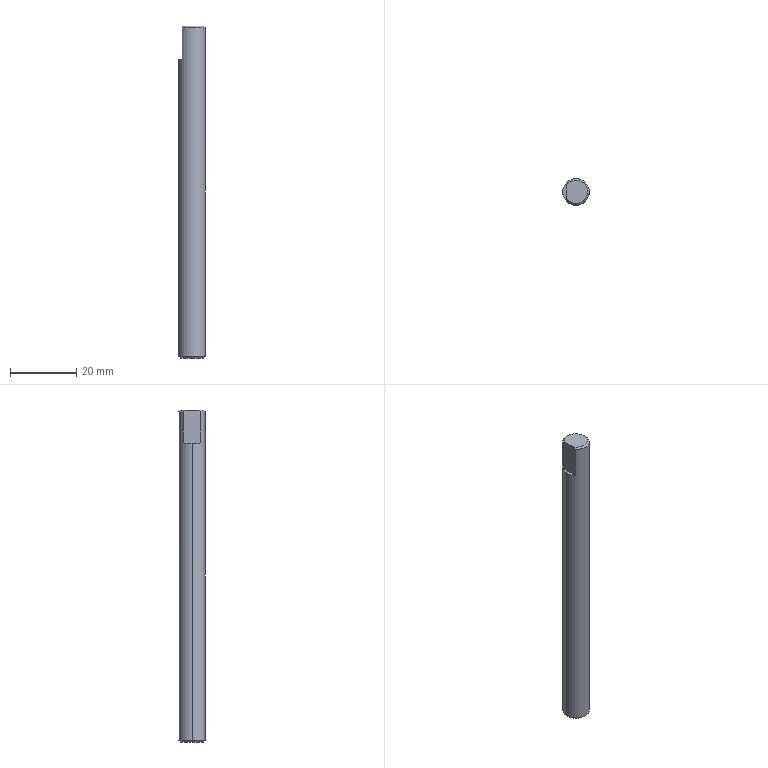Part | STEP file | positioning guide rod | 1 solid | 9 faces | box 8 x 8 x 100 mm | volume 4985 mm3 | plane 4 | cone 3 | cylinder 2 | commonest cylinder face diameters 8 x2
STEP:
#1=CARTESIAN_POINT('',(0.,0.,0.));
#2=DIRECTION('',(0.,0.,1.));
#3=DIRECTION('',(1.,0.,0.));
#4=AXIS2_PLACEMENT_3D('',#1,#2,#3);
#5=CARTESIAN_POINT('',(-3.5,0.,-50.));
#6=VERTEX_POINT('',#5);
#7=CARTESIAN_POINT('',(3.5,0.,-50.));
#8=VERTEX_POINT('',#7);
#9=CARTESIAN_POINT('',(0.,0.,-50.));
#10=DIRECTION('',(0.,0.,-1.));
#11=DIRECTION('',(1.,0.,0.));
#12=AXIS2_PLACEMENT_3D('',#9,#10,#11);
#13=CIRCLE('',#12,3.5);
#14=CARTESIAN_POINT('',(0.,0.,-49.5));
#15=DIRECTION('',(0.,0.,1.));
#16=DIRECTION('',(1.,0.,0.));
#17=AXIS2_PLACEMENT_3D('',#14,#15,#16);
#18=CONICAL_SURFACE('',#17,4.,0.7854);
#19=CARTESIAN_POINT('',(6.283,-0.5));
#20=DIRECTION('',(-1.,0.));
#21=VECTOR('',#20,1.);
#22=LINE('',#19,#21);
#23=(GEOMETRIC_REPRESENTATION_CONTEXT(2)PARAMETRIC_REPRESENTATION_CONTEXT()REPRESENTATION_CONTEXT('',''));
#24=DEFINITIONAL_REPRESENTATION('',(#22),#23);
#25=PCURVE('',#18,#24);
#26=CARTESIAN_POINT('',(0.,0.,-50.));
#27=DIRECTION('',(0.,0.,1.));
#28=DIRECTION('',(1.,0.,0.));
#29=AXIS2_PLACEMENT_3D('',#26,#27,#28);
#30=PLANE('',#29);
#31=CARTESIAN_POINT('',(3.5,0.));
#32=CARTESIAN_POINT('',(3.5,-6.062));
#33=CARTESIAN_POINT('',(-1.75,-3.031));
#34=CARTESIAN_POINT('',(-7.,0.));
#35=CARTESIAN_POINT('',(-1.75,3.031));
#36=CARTESIAN_POINT('',(3.5,6.062));
#37=CARTESIAN_POINT('',(3.5,0.));
#38=(BOUNDED_CURVE()B_SPLINE_CURVE(2,(#31,#32,#33,#34,#35,#36,#37),.UNSPECIFIED.,.T.,.F.)B_SPLINE_CURVE_WITH_KNOTS((1,2,2,2,2,1),(-2.094,0.,2.094,4.189,6.283,8.378),.UNSPECIFIED.)CURVE()GEOMETRIC_REPRESENTATION_ITEM()RATIONAL_B_SPLINE_CURVE((1.,0.5,1.,0.5,1.,0.5,1.))REPRESENTATION_ITEM(''));
#39=(GEOMETRIC_REPRESENTATION_CONTEXT(2)PARAMETRIC_REPRESENTATION_CONTEXT()REPRESENTATION_CONTEXT('',''));
#40=DEFINITIONAL_REPRESENTATION('',(#38),#39);
#41=PCURVE('',#30,#40);
#42=SURFACE_CURVE('',#13,(#25,#41),.PCURVE_S1.);
#43=EDGE_CURVE('',#6,#8,#42,.T.);
#44=ORIENTED_EDGE('',*,*,#43,.F.);
#45=CARTESIAN_POINT('',(-4.,0.,-49.5));
#46=VERTEX_POINT('',#45);
#47=CARTESIAN_POINT('',(-4.,0.,-49.5));
#48=DIRECTION('',(-0.7071,0.,0.7071));
#49=VECTOR('',#48,1.);
#50=LINE('',#47,#49);
#51=CARTESIAN_POINT('',(3.142,0.));
#52=DIRECTION('',(0.,1.));
#53=VECTOR('',#52,1.);
#54=LINE('',#51,#53);
#55=(GEOMETRIC_REPRESENTATION_CONTEXT(2)PARAMETRIC_REPRESENTATION_CONTEXT()REPRESENTATION_CONTEXT('',''));
#56=DEFINITIONAL_REPRESENTATION('',(#54),#55);
#57=PCURVE('',#18,#56);
#58=CARTESIAN_POINT('',(0.,0.,-49.5));
#59=DIRECTION('',(0.,0.,1.));
#60=DIRECTION('',(1.,0.,0.));
#61=AXIS2_PLACEMENT_3D('',#58,#59,#60);
#62=CONICAL_SURFACE('',#61,4.,0.7854);
#63=CARTESIAN_POINT('',(3.142,0.));
#64=DIRECTION('',(0.,1.));
#65=VECTOR('',#64,1.);
#66=LINE('',#63,#65);
#67=(GEOMETRIC_REPRESENTATION_CONTEXT(2)PARAMETRIC_REPRESENTATION_CONTEXT()REPRESENTATION_CONTEXT('',''));
#68=DEFINITIONAL_REPRESENTATION('',(#66),#67);
#69=PCURVE('',#62,#68);
#70=SURFACE_CURVE('',#50,(#57,#69),.PCURVE_S1.);
#71=EDGE_CURVE('',#6,#46,#70,.T.);
#72=ORIENTED_EDGE('',*,*,#71,.T.);
#73=CARTESIAN_POINT('',(4.,0.,-49.5));
#74=VERTEX_POINT('',#73);
#75=CARTESIAN_POINT('',(0.,0.,-49.5));
#76=DIRECTION('',(0.,0.,1.));
#77=DIRECTION('',(1.,0.,0.));
#78=AXIS2_PLACEMENT_3D('',#75,#76,#77);
#79=CIRCLE('',#78,4.);
#80=CARTESIAN_POINT('',(0.,0.));
#81=DIRECTION('',(1.,0.));
#82=VECTOR('',#81,1.);
#83=LINE('',#80,#82);
#84=(GEOMETRIC_REPRESENTATION_CONTEXT(2)PARAMETRIC_REPRESENTATION_CONTEXT()REPRESENTATION_CONTEXT('',''));
#85=DEFINITIONAL_REPRESENTATION('',(#83),#84);
#86=PCURVE('',#18,#85);
#87=CARTESIAN_POINT('',(0.,0.,50.));
#88=DIRECTION('',(0.,0.,-1.));
#89=DIRECTION('',(-1.,0.,0.));
#90=AXIS2_PLACEMENT_3D('',#87,#88,#89);
#91=CYLINDRICAL_SURFACE('',#90,4.);
#92=CARTESIAN_POINT('',(3.142,99.5));
#93=DIRECTION('',(-1.,0.));
#94=VECTOR('',#93,1.);
#95=LINE('',#92,#94);
#96=(GEOMETRIC_REPRESENTATION_CONTEXT(2)PARAMETRIC_REPRESENTATION_CONTEXT()REPRESENTATION_CONTEXT('',''));
#97=DEFINITIONAL_REPRESENTATION('',(#95),#96);
#98=PCURVE('',#91,#97);
#99=SURFACE_CURVE('',#79,(#86,#98),.PCURVE_S1.);
#100=EDGE_CURVE('',#74,#46,#99,.T.);
#101=ORIENTED_EDGE('',*,*,#100,.F.);
#102=CARTESIAN_POINT('',(4.,0.,-49.5));
#103=DIRECTION('',(0.7071,0.,0.7071));
#104=VECTOR('',#103,1.);
#105=LINE('',#102,#104);
#106=CARTESIAN_POINT('',(0.,0.));
#107=DIRECTION('',(0.,1.));
#108=VECTOR('',#107,1.);
#109=LINE('',#106,#108);
#110=(GEOMETRIC_REPRESENTATION_CONTEXT(2)PARAMETRIC_REPRESENTATION_CONTEXT()REPRESENTATION_CONTEXT('',''));
#111=DEFINITIONAL_REPRESENTATION('',(#109),#110);
#112=PCURVE('',#18,#111);
#113=CARTESIAN_POINT('',(6.283,0.));
#114=DIRECTION('',(0.,1.));
#115=VECTOR('',#114,1.);
#116=LINE('',#113,#115);
#117=(GEOMETRIC_REPRESENTATION_CONTEXT(2)PARAMETRIC_REPRESENTATION_CONTEXT()REPRESENTATION_CONTEXT('',''));
#118=DEFINITIONAL_REPRESENTATION('',(#116),#117);
#119=PCURVE('',#62,#118);
#120=SURFACE_CURVE('',#105,(#112,#119),.PCURVE_S1.);
#121=EDGE_CURVE('',#8,#74,#120,.T.);
#122=ORIENTED_EDGE('',*,*,#121,.F.);
#123=EDGE_LOOP('',(#44,#72,#101,#122));
#124=FACE_BOUND('',#123,.T.);
#125=ADVANCED_FACE('',(#124),#18,.T.);
#126=CARTESIAN_POINT('',(-3.,2.646,49.5));
#127=VERTEX_POINT('',#126);
#128=CARTESIAN_POINT('',(4.,0.,49.5));
#129=VERTEX_POINT('',#128);
#130=CARTESIAN_POINT('',(0.,0.,49.5));
#131=DIRECTION('',(0.,0.,-1.));
#132=DIRECTION('',(1.,0.,0.));
#133=AXIS2_PLACEMENT_3D('',#130,#131,#132);
#134=CIRCLE('',#133,4.);
#135=CARTESIAN_POINT('',(-3.142,0.5));
#136=DIRECTION('',(1.,0.));
#137=VECTOR('',#136,1.);
#138=LINE('',#135,#137);
#139=(GEOMETRIC_REPRESENTATION_CONTEXT(2)PARAMETRIC_REPRESENTATION_CONTEXT()REPRESENTATION_CONTEXT('',''));
#140=DEFINITIONAL_REPRESENTATION('',(#138),#139);
#141=PCURVE('',#91,#140);
#142=CARTESIAN_POINT('',(0.,0.,50.));
#143=DIRECTION('',(0.,0.,-1.));
#144=DIRECTION('',(-1.,0.,0.));
#145=AXIS2_PLACEMENT_3D('',#142,#143,#144);
#146=CONICAL_SURFACE('',#145,3.5,0.7854);
#147=CARTESIAN_POINT('',(-3.142,0.5));
#148=DIRECTION('',(1.,0.));
#149=VECTOR('',#148,1.);
#150=LINE('',#147,#149);
#151=(GEOMETRIC_REPRESENTATION_CONTEXT(2)PARAMETRIC_REPRESENTATION_CONTEXT()REPRESENTATION_CONTEXT('',''));
#152=DEFINITIONAL_REPRESENTATION('',(#150),#151);
#153=PCURVE('',#146,#152);
#154=SURFACE_CURVE('',#134,(#141,#153),.PCURVE_S1.);
#155=EDGE_CURVE('',#127,#129,#154,.T.);
#156=ORIENTED_EDGE('',*,*,#155,.T.);
#157=CARTESIAN_POINT('',(4.,0.,50.));
#158=DIRECTION('',(0.,0.,-1.));
#159=VECTOR('',#158,1.);
#160=LINE('',#157,#159);
#161=CARTESIAN_POINT('',(3.142,0.));
#162=DIRECTION('',(0.,1.));
#163=VECTOR('',#162,1.);
#164=LINE('',#161,#163);
#165=(GEOMETRIC_REPRESENTATION_CONTEXT(2)PARAMETRIC_REPRESENTATION_CONTEXT()REPRESENTATION_CONTEXT('',''));
#166=DEFINITIONAL_REPRESENTATION('',(#164),#165);
#167=PCURVE('',#91,#166);
#168=CARTESIAN_POINT('',(0.,0.,50.));
#169=DIRECTION('',(0.,0.,-1.));
#170=DIRECTION('',(-1.,0.,0.));
#171=AXIS2_PLACEMENT_3D('',#168,#169,#170);
#172=CYLINDRICAL_SURFACE('',#171,4.);
#173=CARTESIAN_POINT('',(3.142,0.));
#174=DIRECTION('',(0.,1.));
#175=VECTOR('',#174,1.);
#176=LINE('',#173,#175);
#177=(GEOMETRIC_REPRESENTATION_CONTEXT(2)PARAMETRIC_REPRESENTATION_CONTEXT()REPRESENTATION_CONTEXT('',''));
#178=DEFINITIONAL_REPRESENTATION('',(#176),#177);
#179=PCURVE('',#172,#178);
#180=SURFACE_CURVE('',#160,(#167,#179),.PCURVE_S1.);
#181=EDGE_CURVE('',#129,#74,#180,.T.);
#182=ORIENTED_EDGE('',*,*,#181,.T.);
#183=ORIENTED_EDGE('',*,*,#100,.T.);
#184=CARTESIAN_POINT('',(-4.,0.,40.));
#185=VERTEX_POINT('',#184);
#186=CARTESIAN_POINT('',(-4.,0.,50.));
#187=DIRECTION('',(0.,0.,-1.));
#188=VECTOR('',#187,1.);
#189=LINE('',#186,#188);
#190=CARTESIAN_POINT('',(0.,0.));
#191=DIRECTION('',(0.,1.));
#192=VECTOR('',#191,1.);
#193=LINE('',#190,#192);
#194=(GEOMETRIC_REPRESENTATION_CONTEXT(2)PARAMETRIC_REPRESENTATION_CONTEXT()REPRESENTATION_CONTEXT('',''));
#195=DEFINITIONAL_REPRESENTATION('',(#193),#194);
#196=PCURVE('',#91,#195);
#197=CARTESIAN_POINT('',(6.283,0.));
#198=DIRECTION('',(0.,1.));
#199=VECTOR('',#198,1.);
#200=LINE('',#197,#199);
#201=(GEOMETRIC_REPRESENTATION_CONTEXT(2)PARAMETRIC_REPRESENTATION_CONTEXT()REPRESENTATION_CONTEXT('',''));
#202=DEFINITIONAL_REPRESENTATION('',(#200),#201);
#203=PCURVE('',#172,#202);
#204=SURFACE_CURVE('',#189,(#196,#203),.PCURVE_S1.);
#205=EDGE_CURVE('',#185,#46,#204,.T.);
#206=ORIENTED_EDGE('',*,*,#205,.F.);
#207=CARTESIAN_POINT('',(-3.,2.646,40.));
#208=VERTEX_POINT('',#207);
#209=CARTESIAN_POINT('',(0.,0.,40.));
#210=DIRECTION('',(0.,0.,1.));
#211=DIRECTION('',(1.,0.,0.));
#212=AXIS2_PLACEMENT_3D('',#209,#210,#211);
#213=CIRCLE('',#212,4.);
#214=CARTESIAN_POINT('',(3.142,10.));
#215=DIRECTION('',(-1.,0.));
#216=VECTOR('',#215,1.);
#217=LINE('',#214,#216);
#218=(GEOMETRIC_REPRESENTATION_CONTEXT(2)PARAMETRIC_REPRESENTATION_CONTEXT()REPRESENTATION_CONTEXT('',''));
#219=DEFINITIONAL_REPRESENTATION('',(#217),#218);
#220=PCURVE('',#91,#219);
#221=CARTESIAN_POINT('',(0.,0.,40.));
#222=DIRECTION('',(0.,0.,1.));
#223=DIRECTION('',(1.,0.,0.));
#224=AXIS2_PLACEMENT_3D('',#221,#222,#223);
#225=PLANE('',#224);
#226=CARTESIAN_POINT('',(0.,0.));
#227=DIRECTION('',(1.,0.));
#228=AXIS2_PLACEMENT_2D('',#226,#227);
#229=CIRCLE('',#228,4.);
#230=(GEOMETRIC_REPRESENTATION_CONTEXT(2)PARAMETRIC_REPRESENTATION_CONTEXT()REPRESENTATION_CONTEXT('',''));
#231=DEFINITIONAL_REPRESENTATION('',(#229),#230);
#232=PCURVE('',#225,#231);
#233=SURFACE_CURVE('',#213,(#220,#232),.PCURVE_S1.);
#234=EDGE_CURVE('',#208,#185,#233,.T.);
#235=ORIENTED_EDGE('',*,*,#234,.F.);
#236=CARTESIAN_POINT('',(-3.,2.646,50.));
#237=DIRECTION('',(0.,0.,1.));
#238=VECTOR('',#237,1.);
#239=LINE('',#236,#238);
#240=CARTESIAN_POINT('',(0.7227,0.));
#241=DIRECTION('',(0.,-1.));
#242=VECTOR('',#241,1.);
#243=LINE('',#240,#242);
#244=(GEOMETRIC_REPRESENTATION_CONTEXT(2)PARAMETRIC_REPRESENTATION_CONTEXT()REPRESENTATION_CONTEXT('',''));
#245=DEFINITIONAL_REPRESENTATION('',(#243),#244);
#246=PCURVE('',#91,#245);
#247=CARTESIAN_POINT('',(-3.,2.975,40.));
#248=DIRECTION('',(1.,0.,0.));
#249=DIRECTION('',(0.,1.,0.));
#250=AXIS2_PLACEMENT_3D('',#247,#248,#249);
#251=PLANE('',#250);
#252=CARTESIAN_POINT('',(-0.329,10.));
#253=DIRECTION('',(0.,1.));
#254=VECTOR('',#253,1.);
#255=LINE('',#252,#254);
#256=(GEOMETRIC_REPRESENTATION_CONTEXT(2)PARAMETRIC_REPRESENTATION_CONTEXT()REPRESENTATION_CONTEXT('',''));
#257=DEFINITIONAL_REPRESENTATION('',(#255),#256);
#258=PCURVE('',#251,#257);
#259=SURFACE_CURVE('',#239,(#246,#258),.PCURVE_S1.);
#260=EDGE_CURVE('',#208,#127,#259,.T.);
#261=ORIENTED_EDGE('',*,*,#260,.T.);
#262=EDGE_LOOP('',(#156,#182,#183,#206,#235,#261));
#263=FACE_BOUND('',#262,.T.);
#264=ADVANCED_FACE('',(#263),#91,.T.);
#265=ORIENTED_EDGE('',*,*,#181,.F.);
#266=CARTESIAN_POINT('',(-3.,-2.646,49.5));
#267=VERTEX_POINT('',#266);
#268=CARTESIAN_POINT('',(0.,0.,49.5));
#269=DIRECTION('',(0.,0.,-1.));
#270=DIRECTION('',(1.,0.,0.));
#271=AXIS2_PLACEMENT_3D('',#268,#269,#270);
#272=CIRCLE('',#271,4.);
#273=CARTESIAN_POINT('',(3.142,0.5));
#274=DIRECTION('',(1.,0.));
#275=VECTOR('',#274,1.);
#276=LINE('',#273,#275);
#277=(GEOMETRIC_REPRESENTATION_CONTEXT(2)PARAMETRIC_REPRESENTATION_CONTEXT()REPRESENTATION_CONTEXT('',''));
#278=DEFINITIONAL_REPRESENTATION('',(#276),#277);
#279=PCURVE('',#172,#278);
#280=CARTESIAN_POINT('',(3.142,0.5));
#281=DIRECTION('',(1.,0.));
#282=VECTOR('',#281,1.);
#283=LINE('',#280,#282);
#284=(GEOMETRIC_REPRESENTATION_CONTEXT(2)PARAMETRIC_REPRESENTATION_CONTEXT()REPRESENTATION_CONTEXT('',''));
#285=DEFINITIONAL_REPRESENTATION('',(#283),#284);
#286=PCURVE('',#146,#285);
#287=SURFACE_CURVE('',#272,(#279,#286),.PCURVE_S1.);
#288=EDGE_CURVE('',#129,#267,#287,.T.);
#289=ORIENTED_EDGE('',*,*,#288,.T.);
#290=CARTESIAN_POINT('',(-3.,-2.646,40.));
#291=VERTEX_POINT('',#290);
#292=CARTESIAN_POINT('',(-3.,-2.646,50.));
#293=DIRECTION('',(0.,0.,-1.));
#294=VECTOR('',#293,1.);
#295=LINE('',#292,#294);
#296=CARTESIAN_POINT('',(5.56,0.));
#297=DIRECTION('',(0.,1.));
#298=VECTOR('',#297,1.);
#299=LINE('',#296,#298);
#300=(GEOMETRIC_REPRESENTATION_CONTEXT(2)PARAMETRIC_REPRESENTATION_CONTEXT()REPRESENTATION_CONTEXT('',''));
#301=DEFINITIONAL_REPRESENTATION('',(#299),#300);
#302=PCURVE('',#172,#301);
#303=CARTESIAN_POINT('',(-5.62,10.));
#304=DIRECTION('',(0.,-1.));
#305=VECTOR('',#304,1.);
#306=LINE('',#303,#305);
#307=(GEOMETRIC_REPRESENTATION_CONTEXT(2)PARAMETRIC_REPRESENTATION_CONTEXT()REPRESENTATION_CONTEXT('',''));
#308=DEFINITIONAL_REPRESENTATION('',(#306),#307);
#309=PCURVE('',#251,#308);
#310=SURFACE_CURVE('',#295,(#302,#309),.PCURVE_S1.);
#311=EDGE_CURVE('',#267,#291,#310,.T.);
#312=ORIENTED_EDGE('',*,*,#311,.T.);
#313=CARTESIAN_POINT('',(0.,0.,40.));
#314=DIRECTION('',(0.,0.,1.));
#315=DIRECTION('',(1.,0.,0.));
#316=AXIS2_PLACEMENT_3D('',#313,#314,#315);
#317=CIRCLE('',#316,4.);
#318=CARTESIAN_POINT('',(9.425,10.));
#319=DIRECTION('',(-1.,0.));
#320=VECTOR('',#319,1.);
#321=LINE('',#318,#320);
#322=(GEOMETRIC_REPRESENTATION_CONTEXT(2)PARAMETRIC_REPRESENTATION_CONTEXT()REPRESENTATION_CONTEXT('',''));
#323=DEFINITIONAL_REPRESENTATION('',(#321),#322);
#324=PCURVE('',#172,#323);
#325=CARTESIAN_POINT('',(0.,0.));
#326=DIRECTION('',(1.,0.));
#327=AXIS2_PLACEMENT_2D('',#325,#326);
#328=CIRCLE('',#327,4.);
#329=(GEOMETRIC_REPRESENTATION_CONTEXT(2)PARAMETRIC_REPRESENTATION_CONTEXT()REPRESENTATION_CONTEXT('',''));
#330=DEFINITIONAL_REPRESENTATION('',(#328),#329);
#331=PCURVE('',#225,#330);
#332=SURFACE_CURVE('',#317,(#324,#331),.PCURVE_S1.);
#333=EDGE_CURVE('',#185,#291,#332,.T.);
#334=ORIENTED_EDGE('',*,*,#333,.F.);
#335=ORIENTED_EDGE('',*,*,#205,.T.);
#336=CARTESIAN_POINT('',(0.,0.,-49.5));
#337=DIRECTION('',(0.,0.,1.));
#338=DIRECTION('',(1.,0.,0.));
#339=AXIS2_PLACEMENT_3D('',#336,#337,#338);
#340=CIRCLE('',#339,4.);
#341=CARTESIAN_POINT('',(9.425,99.5));
#342=DIRECTION('',(-1.,0.));
#343=VECTOR('',#342,1.);
#344=LINE('',#341,#343);
#345=(GEOMETRIC_REPRESENTATION_CONTEXT(2)PARAMETRIC_REPRESENTATION_CONTEXT()REPRESENTATION_CONTEXT('',''));
#346=DEFINITIONAL_REPRESENTATION('',(#344),#345);
#347=PCURVE('',#172,#346);
#348=CARTESIAN_POINT('',(0.,0.));
#349=DIRECTION('',(1.,0.));
#350=VECTOR('',#349,1.);
#351=LINE('',#348,#350);
#352=(GEOMETRIC_REPRESENTATION_CONTEXT(2)PARAMETRIC_REPRESENTATION_CONTEXT()REPRESENTATION_CONTEXT('',''));
#353=DEFINITIONAL_REPRESENTATION('',(#351),#352);
#354=PCURVE('',#62,#353);
#355=SURFACE_CURVE('',#340,(#347,#354),.PCURVE_S1.);
#356=EDGE_CURVE('',#46,#74,#355,.T.);
#357=ORIENTED_EDGE('',*,*,#356,.T.);
#358=EDGE_LOOP('',(#265,#289,#312,#334,#335,#357));
#359=FACE_BOUND('',#358,.T.);
#360=ADVANCED_FACE('',(#359),#172,.T.);
#361=CARTESIAN_POINT('',(-3.,-1.803,50.));
#362=VERTEX_POINT('',#361);
#363=CARTESIAN_POINT('',(-3.,1.803,50.));
#364=VERTEX_POINT('',#363);
#365=CARTESIAN_POINT('',(-3.,2.975,50.));
#366=DIRECTION('',(0.,1.,0.));
#367=VECTOR('',#366,1.);
#368=LINE('',#365,#367);
#369=CARTESIAN_POINT('',(0.,0.,50.));
#370=DIRECTION('',(0.,0.,1.));
#371=DIRECTION('',(1.,0.,0.));
#372=AXIS2_PLACEMENT_3D('',#369,#370,#371);
#373=PLANE('',#372);
#374=CARTESIAN_POINT('',(-3.,2.975));
#375=DIRECTION('',(0.,1.));
#376=VECTOR('',#375,1.);
#377=LINE('',#374,#376);
#378=(GEOMETRIC_REPRESENTATION_CONTEXT(2)PARAMETRIC_REPRESENTATION_CONTEXT()REPRESENTATION_CONTEXT('',''));
#379=DEFINITIONAL_REPRESENTATION('',(#377),#378);
#380=PCURVE('',#373,#379);
#381=CARTESIAN_POINT('',(0.,10.));
#382=DIRECTION('',(1.,0.));
#383=VECTOR('',#382,1.);
#384=LINE('',#381,#383);
#385=(GEOMETRIC_REPRESENTATION_CONTEXT(2)PARAMETRIC_REPRESENTATION_CONTEXT()REPRESENTATION_CONTEXT('',''));
#386=DEFINITIONAL_REPRESENTATION('',(#384),#385);
#387=PCURVE('',#251,#386);
#388=SURFACE_CURVE('',#368,(#380,#387),.PCURVE_S1.);
#389=EDGE_CURVE('',#362,#364,#388,.T.);
#390=ORIENTED_EDGE('',*,*,#389,.F.);
#391=CARTESIAN_POINT('',(0.,0.,50.));
#392=DIRECTION('',(0.,0.,1.));
#393=DIRECTION('',(1.,0.,0.));
#394=AXIS2_PLACEMENT_3D('',#391,#392,#393);
#395=CIRCLE('',#394,3.5);
#396=CARTESIAN_POINT('',(0.,0.));
#397=DIRECTION('',(1.,0.));
#398=AXIS2_PLACEMENT_2D('',#396,#397);
#399=CIRCLE('',#398,3.5);
#400=(GEOMETRIC_REPRESENTATION_CONTEXT(2)PARAMETRIC_REPRESENTATION_CONTEXT()REPRESENTATION_CONTEXT('',''));
#401=DEFINITIONAL_REPRESENTATION('',(#399),#400);
#402=PCURVE('',#373,#401);
#403=CARTESIAN_POINT('',(9.425,0.));
#404=DIRECTION('',(-1.,0.));
#405=VECTOR('',#404,1.);
#406=LINE('',#403,#405);
#407=(GEOMETRIC_REPRESENTATION_CONTEXT(2)PARAMETRIC_REPRESENTATION_CONTEXT()REPRESENTATION_CONTEXT('',''));
#408=DEFINITIONAL_REPRESENTATION('',(#406),#407);
#409=PCURVE('',#146,#408);
#410=SURFACE_CURVE('',#395,(#402,#409),.PCURVE_S1.);
#411=EDGE_CURVE('',#362,#364,#410,.T.);
#412=ORIENTED_EDGE('',*,*,#411,.T.);
#413=EDGE_LOOP('',(#390,#412));
#414=FACE_BOUND('',#413,.T.);
#415=ADVANCED_FACE('',(#414),#373,.T.);
#416=CARTESIAN_POINT('',(0.,0.,-50.));
#417=DIRECTION('',(0.,0.,-1.));
#418=DIRECTION('',(1.,0.,0.));
#419=AXIS2_PLACEMENT_3D('',#416,#417,#418);
#420=CIRCLE('',#419,3.5);
#421=CARTESIAN_POINT('',(3.5,0.));
#422=CARTESIAN_POINT('',(3.5,-6.062));
#423=CARTESIAN_POINT('',(-1.75,-3.031));
#424=CARTESIAN_POINT('',(-7.,0.));
#425=CARTESIAN_POINT('',(-1.75,3.031));
#426=CARTESIAN_POINT('',(3.5,6.062));
#427=CARTESIAN_POINT('',(3.5,0.));
#428=(BOUNDED_CURVE()B_SPLINE_CURVE(2,(#421,#422,#423,#424,#425,#426,#427),.UNSPECIFIED.,.T.,.F.)B_SPLINE_CURVE_WITH_KNOTS((1,2,2,2,2,1),(-2.094,0.,2.094,4.189,6.283,8.378),.UNSPECIFIED.)CURVE()GEOMETRIC_REPRESENTATION_ITEM()RATIONAL_B_SPLINE_CURVE((1.,0.5,1.,0.5,1.,0.5,1.))REPRESENTATION_ITEM(''));
#429=(GEOMETRIC_REPRESENTATION_CONTEXT(2)PARAMETRIC_REPRESENTATION_CONTEXT()REPRESENTATION_CONTEXT('',''));
#430=DEFINITIONAL_REPRESENTATION('',(#428),#429);
#431=PCURVE('',#30,#430);
#432=CARTESIAN_POINT('',(6.283,-0.5));
#433=DIRECTION('',(-1.,0.));
#434=VECTOR('',#433,1.);
#435=LINE('',#432,#434);
#436=(GEOMETRIC_REPRESENTATION_CONTEXT(2)PARAMETRIC_REPRESENTATION_CONTEXT()REPRESENTATION_CONTEXT('',''));
#437=DEFINITIONAL_REPRESENTATION('',(#435),#436);
#438=PCURVE('',#62,#437);
#439=SURFACE_CURVE('',#420,(#431,#438),.PCURVE_S1.);
#440=EDGE_CURVE('',#8,#6,#439,.T.);
#441=ORIENTED_EDGE('',*,*,#440,.T.);
#442=ORIENTED_EDGE('',*,*,#43,.T.);
#443=EDGE_LOOP('',(#441,#442));
#444=FACE_BOUND('',#443,.T.);
#445=ADVANCED_FACE('',(#444),#30,.F.);
#446=ORIENTED_EDGE('',*,*,#71,.F.);
#447=ORIENTED_EDGE('',*,*,#440,.F.);
#448=ORIENTED_EDGE('',*,*,#121,.T.);
#449=ORIENTED_EDGE('',*,*,#356,.F.);
#450=EDGE_LOOP('',(#446,#447,#448,#449));
#451=FACE_BOUND('',#450,.T.);
#452=ADVANCED_FACE('',(#451),#62,.T.);
#453=CARTESIAN_POINT('',(-3.,-2.646,49.5));
#454=CARTESIAN_POINT('',(-3.,-2.373,49.68));
#455=CARTESIAN_POINT('',(-3.,-2.093,49.851));
#456=CARTESIAN_POINT('',(-3.,-1.803,50.));
#457=B_SPLINE_CURVE_WITH_KNOTS('',3,(#453,#454,#455,#456),.UNSPECIFIED.,.F.,.F.,(4,4),(0.006163,0.007143),.PIECEWISE_BEZIER_KNOTS.);
#458=CARTESIAN_POINT('',(5.56,0.5));
#459=CARTESIAN_POINT('',(5.563,0.4918));
#460=CARTESIAN_POINT('',(5.567,0.4755));
#461=CARTESIAN_POINT('',(5.575,0.4511));
#462=CARTESIAN_POINT('',(5.582,0.4268));
#463=CARTESIAN_POINT('',(5.589,0.4027));
#464=CARTESIAN_POINT('',(5.597,0.3788));
#465=CARTESIAN_POINT('',(5.604,0.355));
#466=CARTESIAN_POINT('',(5.612,0.3313));
#467=CARTESIAN_POINT('',(5.62,0.3078));
#468=CARTESIAN_POINT('',(5.628,0.2845));
#469=CARTESIAN_POINT('',(5.636,0.2614));
#470=CARTESIAN_POINT('',(5.644,0.2384));
#471=CARTESIAN_POINT('',(5.652,0.2157));
#472=CARTESIAN_POINT('',(5.66,0.1931));
#473=CARTESIAN_POINT('',(5.669,0.1707));
#474=CARTESIAN_POINT('',(5.678,0.1486));
#475=CARTESIAN_POINT('',(5.686,0.1266));
#476=CARTESIAN_POINT('',(5.695,0.1049));
#477=CARTESIAN_POINT('',(5.704,0.08345));
#478=CARTESIAN_POINT('',(5.714,0.0622));
#479=CARTESIAN_POINT('',(5.723,0.0412));
#480=CARTESIAN_POINT('',(5.732,0.02045));
#481=CARTESIAN_POINT('',(5.739,0.006787));
#482=CARTESIAN_POINT('',(5.742,0.));
#483=B_SPLINE_CURVE_WITH_KNOTS('',3,(#458,#459,#460,#461,#462,#463,#464,#465,#466,#467,#468,#469,#470,#471,#472,#473,#474,#475,#476,#477,#478,#479,#480,#481,#482),.UNSPECIFIED.,.F.,.F.,(4,1,1,1,1,1,1,1,1,1,1,1,1,1,1,1,1,1,1,1,1,1,4),(0.006163,0.006208,0.006252,0.006297,0.006341,0.006386,0.00643,0.006475,0.006519,0.006564,0.006608,0.006653,0.006697,0.006742,0.006787,0.006831,0.006876,0.00692,0.006965,0.007009,0.007054,0.007098,0.007143),.QUASI_UNIFORM_KNOTS.);
#484=(GEOMETRIC_REPRESENTATION_CONTEXT(2)PARAMETRIC_REPRESENTATION_CONTEXT()REPRESENTATION_CONTEXT('',''));
#485=DEFINITIONAL_REPRESENTATION('',(#483),#484);
#486=PCURVE('',#146,#485);
#487=CARTESIAN_POINT('',(-5.62,9.5));
#488=CARTESIAN_POINT('',(-5.348,9.68));
#489=CARTESIAN_POINT('',(-5.067,9.851));
#490=CARTESIAN_POINT('',(-4.778,10.));
#491=B_SPLINE_CURVE_WITH_KNOTS('',3,(#487,#488,#489,#490),.UNSPECIFIED.,.F.,.F.,(4,4),(0.006163,0.007143),.PIECEWISE_BEZIER_KNOTS.);
#492=(GEOMETRIC_REPRESENTATION_CONTEXT(2)PARAMETRIC_REPRESENTATION_CONTEXT()REPRESENTATION_CONTEXT('',''));
#493=DEFINITIONAL_REPRESENTATION('',(#491),#492);
#494=PCURVE('',#251,#493);
#495=SURFACE_CURVE('',#457,(#486,#494),.PCURVE_S1.);
#496=EDGE_CURVE('',#267,#362,#495,.T.);
#497=ORIENTED_EDGE('',*,*,#496,.F.);
#498=ORIENTED_EDGE('',*,*,#288,.F.);
#499=ORIENTED_EDGE('',*,*,#155,.F.);
#500=CARTESIAN_POINT('',(-3.,1.803,50.));
#501=CARTESIAN_POINT('',(-3.,2.093,49.85));
#502=CARTESIAN_POINT('',(-3.,2.373,49.681));
#503=CARTESIAN_POINT('',(-3.,2.646,49.5));
#504=B_SPLINE_CURVE_WITH_KNOTS('',3,(#500,#501,#502,#503),.UNSPECIFIED.,.F.,.F.,(4,4),(0.01093,0.01192),.PIECEWISE_BEZIER_KNOTS.);
#505=CARTESIAN_POINT('',(0.5411,0.));
#506=CARTESIAN_POINT('',(0.5443,0.006806));
#507=CARTESIAN_POINT('',(0.5508,0.0205));
#508=CARTESIAN_POINT('',(0.5602,0.04129));
#509=CARTESIAN_POINT('',(0.5696,0.06232));
#510=CARTESIAN_POINT('',(0.5788,0.08358));
#511=CARTESIAN_POINT('',(0.5879,0.1051));
#512=CARTESIAN_POINT('',(0.5968,0.1268));
#513=CARTESIAN_POINT('',(0.6056,0.1487));
#514=CARTESIAN_POINT('',(0.6142,0.1708));
#515=CARTESIAN_POINT('',(0.6228,0.1932));
#516=CARTESIAN_POINT('',(0.6312,0.2157));
#517=CARTESIAN_POINT('',(0.6394,0.2385));
#518=CARTESIAN_POINT('',(0.6476,0.2614));
#519=CARTESIAN_POINT('',(0.6556,0.2845));
#520=CARTESIAN_POINT('',(0.6635,0.3078));
#521=CARTESIAN_POINT('',(0.6713,0.3312));
#522=CARTESIAN_POINT('',(0.679,0.3549));
#523=CARTESIAN_POINT('',(0.6866,0.3787));
#524=CARTESIAN_POINT('',(0.694,0.4026));
#525=CARTESIAN_POINT('',(0.7013,0.4267));
#526=CARTESIAN_POINT('',(0.7086,0.451));
#527=CARTESIAN_POINT('',(0.7157,0.4754));
#528=CARTESIAN_POINT('',(0.7204,0.4918));
#529=CARTESIAN_POINT('',(0.7227,0.5));
#530=B_SPLINE_CURVE_WITH_KNOTS('',3,(#505,#506,#507,#508,#509,#510,#511,#512,#513,#514,#515,#516,#517,#518,#519,#520,#521,#522,#523,#524,#525,#526,#527,#528,#529),.UNSPECIFIED.,.F.,.F.,(4,1,1,1,1,1,1,1,1,1,1,1,1,1,1,1,1,1,1,1,1,1,4),(0.01093,0.01097,0.01102,0.01106,0.01111,0.01115,0.0112,0.01124,0.01129,0.01133,0.01138,0.01142,0.01147,0.01151,0.01156,0.0116,0.01165,0.01169,0.01174,0.01178,0.01183,0.01187,0.01192),.QUASI_UNIFORM_KNOTS.);
#531=(GEOMETRIC_REPRESENTATION_CONTEXT(2)PARAMETRIC_REPRESENTATION_CONTEXT()REPRESENTATION_CONTEXT('',''));
#532=DEFINITIONAL_REPRESENTATION('',(#530),#531);
#533=PCURVE('',#146,#532);
#534=CARTESIAN_POINT('',(-1.172,10.));
#535=CARTESIAN_POINT('',(-0.8813,9.85));
#536=CARTESIAN_POINT('',(-0.602,9.681));
#537=CARTESIAN_POINT('',(-0.329,9.5));
#538=B_SPLINE_CURVE_WITH_KNOTS('',3,(#534,#535,#536,#537),.UNSPECIFIED.,.F.,.F.,(4,4),(0.01093,0.01192),.PIECEWISE_BEZIER_KNOTS.);
#539=(GEOMETRIC_REPRESENTATION_CONTEXT(2)PARAMETRIC_REPRESENTATION_CONTEXT()REPRESENTATION_CONTEXT('',''));
#540=DEFINITIONAL_REPRESENTATION('',(#538),#539);
#541=PCURVE('',#251,#540);
#542=SURFACE_CURVE('',#504,(#533,#541),.PCURVE_S1.);
#543=EDGE_CURVE('',#364,#127,#542,.T.);
#544=ORIENTED_EDGE('',*,*,#543,.F.);
#545=ORIENTED_EDGE('',*,*,#411,.F.);
#546=EDGE_LOOP('',(#497,#498,#499,#544,#545));
#547=FACE_BOUND('',#546,.T.);
#548=ADVANCED_FACE('',(#547),#146,.T.);
#549=ORIENTED_EDGE('',*,*,#234,.T.);
#550=ORIENTED_EDGE('',*,*,#333,.T.);
#551=CARTESIAN_POINT('',(-3.,2.975,40.));
#552=DIRECTION('',(0.,1.,0.));
#553=VECTOR('',#552,1.);
#554=LINE('',#551,#553);
#555=CARTESIAN_POINT('',(-3.,2.975));
#556=DIRECTION('',(0.,1.));
#557=VECTOR('',#556,1.);
#558=LINE('',#555,#557);
#559=(GEOMETRIC_REPRESENTATION_CONTEXT(2)PARAMETRIC_REPRESENTATION_CONTEXT()REPRESENTATION_CONTEXT('',''));
#560=DEFINITIONAL_REPRESENTATION('',(#558),#559);
#561=PCURVE('',#225,#560);
#562=CARTESIAN_POINT('',(0.,0.));
#563=DIRECTION('',(1.,0.));
#564=VECTOR('',#563,1.);
#565=LINE('',#562,#564);
#566=(GEOMETRIC_REPRESENTATION_CONTEXT(2)PARAMETRIC_REPRESENTATION_CONTEXT()REPRESENTATION_CONTEXT('',''));
#567=DEFINITIONAL_REPRESENTATION('',(#565),#566);
#568=PCURVE('',#251,#567);
#569=SURFACE_CURVE('',#554,(#561,#568),.PCURVE_S1.);
#570=EDGE_CURVE('',#291,#208,#569,.T.);
#571=ORIENTED_EDGE('',*,*,#570,.T.);
#572=EDGE_LOOP('',(#549,#550,#571));
#573=FACE_BOUND('',#572,.T.);
#574=ADVANCED_FACE('',(#573),#225,.T.);
#575=ORIENTED_EDGE('',*,*,#496,.T.);
#576=ORIENTED_EDGE('',*,*,#389,.T.);
#577=ORIENTED_EDGE('',*,*,#543,.T.);
#578=ORIENTED_EDGE('',*,*,#260,.F.);
#579=ORIENTED_EDGE('',*,*,#570,.F.);
#580=ORIENTED_EDGE('',*,*,#311,.F.);
#581=EDGE_LOOP('',(#575,#576,#577,#578,#579,#580));
#582=FACE_BOUND('',#581,.T.);
#583=ADVANCED_FACE('',(#582),#251,.F.);
#584=CLOSED_SHELL('',(#125,#264,#360,#415,#445,#452,#548,#574,#583));
#585=MANIFOLD_SOLID_BREP('',#584);
#586=(LENGTH_UNIT()NAMED_UNIT(*)SI_UNIT(.MILLI.,.METRE.));
#587=UNCERTAINTY_MEASURE_WITH_UNIT(LENGTH_MEASURE(0.00002),#586,'','');
#588=(NAMED_UNIT(*)PLANE_ANGLE_UNIT()SI_UNIT($,.RADIAN.));
#589=(NAMED_UNIT(*)SI_UNIT($,.STERADIAN.)SOLID_ANGLE_UNIT());
#590=(GEOMETRIC_REPRESENTATION_CONTEXT(3)GLOBAL_UNCERTAINTY_ASSIGNED_CONTEXT((#587))GLOBAL_UNIT_ASSIGNED_CONTEXT((#586,#588,#589))REPRESENTATION_CONTEXT('',''));
#591=ADVANCED_BREP_SHAPE_REPRESENTATION('',(#4,#585),#590);